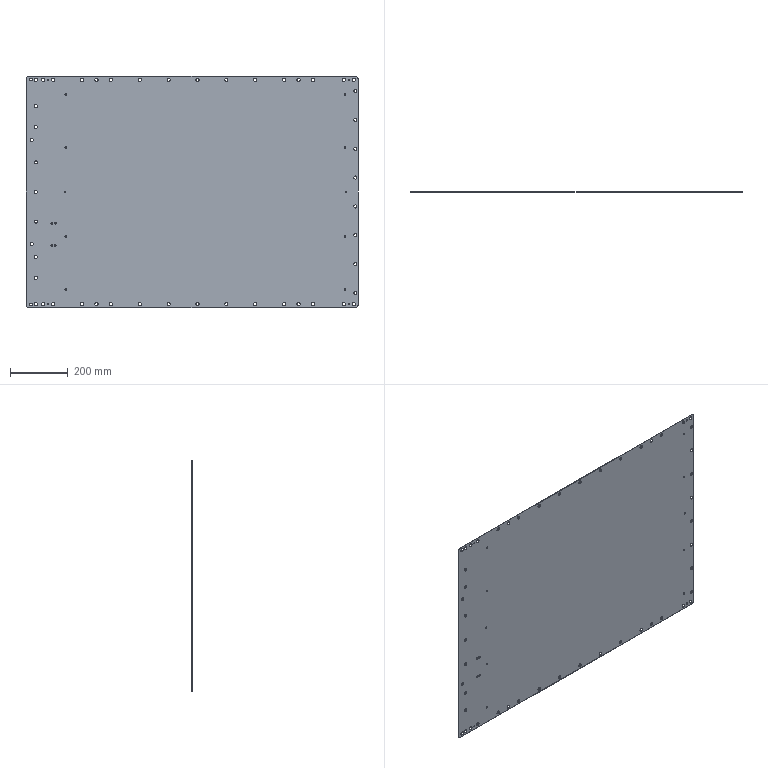Part | NX | features BREP 1 | 1 solid | 152 faces | box 1150 x 1.2 x 803 mm | volume 1101671 mm3 | cylinder 142 | plane 10 | commonest cylinder face diameters 11 x94 6 x28 4.1 x8 10 x4 10.5 x4 20 x4